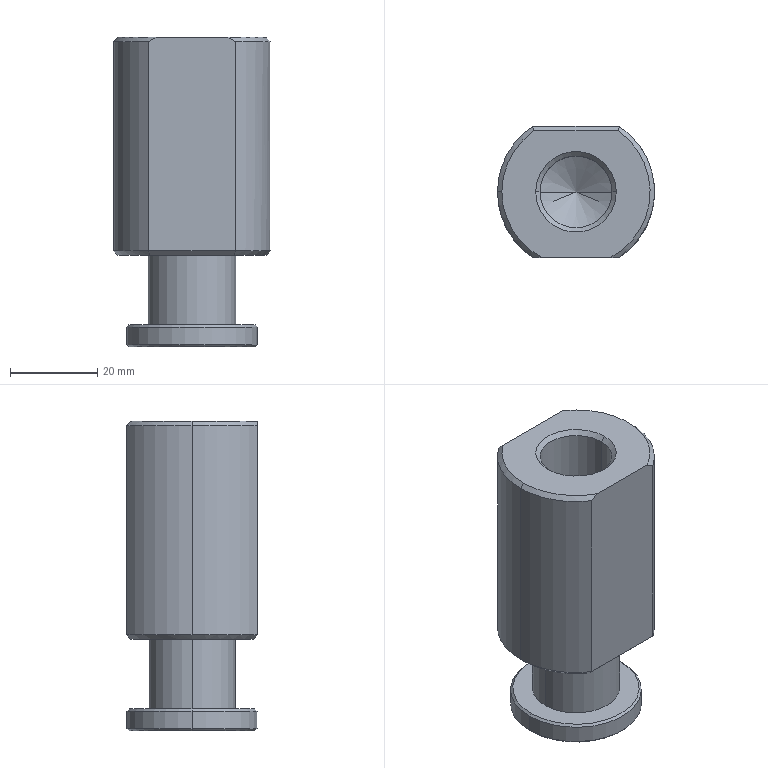Part | STEP file | YCD14007A-08.02.11 Horizontal Cylinder Joint | 1 solid | 32 faces | box 36 x 30 x 71 mm | volume 47737 mm3 | cone 14 | cylinder 9 | plane 9 | commonest cylinder face diameters 36 x3 16.5 x2 20 x2 30 x2